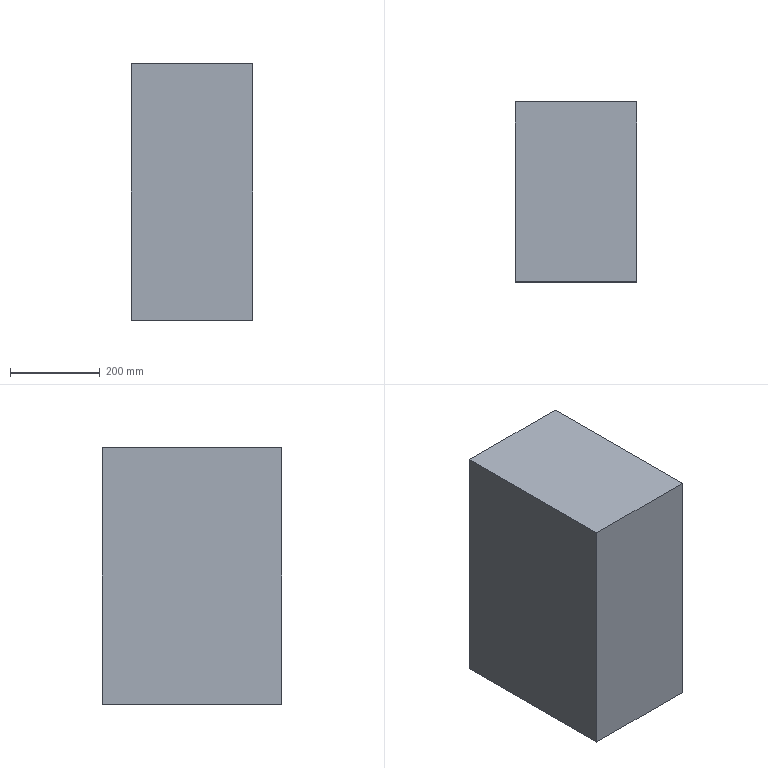Part | STEP file | kunzaxiang | 1 solid | 11 faces | box 270 x 400 x 570 mm | volume 12312000 mm3 | plane 11
STEP:
#1=CARTESIAN_POINT('',(0.,0.,0.));
#2=DIRECTION('',(0.,0.,1.));
#3=DIRECTION('',(1.,0.,0.));
#4=AXIS2_PLACEMENT_3D('',#1,#2,#3);
#5=CARTESIAN_POINT('',(135.,200.,285.));
#6=VERTEX_POINT('',#5);
#7=CARTESIAN_POINT('',(135.,200.,-285.));
#8=VERTEX_POINT('',#7);
#9=CARTESIAN_POINT('',(135.,200.,-285.));
#10=DIRECTION('',(0.,0.,-1.));
#11=VECTOR('',#10,1.);
#12=LINE('',#9,#11);
#13=CARTESIAN_POINT('',(0.,200.,0.));
#14=DIRECTION('',(0.,1.,0.));
#15=DIRECTION('',(0.,0.,1.));
#16=AXIS2_PLACEMENT_3D('',#13,#14,#15);
#17=PLANE('',#16);
#18=CARTESIAN_POINT('',(-285.,135.));
#19=DIRECTION('',(-1.,0.));
#20=VECTOR('',#19,1.);
#21=LINE('',#18,#20);
#22=(GEOMETRIC_REPRESENTATION_CONTEXT(2)PARAMETRIC_REPRESENTATION_CONTEXT()REPRESENTATION_CONTEXT('',''));
#23=DEFINITIONAL_REPRESENTATION('',(#21),#22);
#24=PCURVE('',#17,#23);
#25=CARTESIAN_POINT('',(135.,-200.,-285.));
#26=DIRECTION('',(1.,0.,0.));
#27=DIRECTION('',(0.,0.,-1.));
#28=AXIS2_PLACEMENT_3D('',#25,#26,#27);
#29=PLANE('',#28);
#30=CARTESIAN_POINT('',(0.,400.));
#31=DIRECTION('',(1.,0.));
#32=VECTOR('',#31,1.);
#33=LINE('',#30,#32);
#34=(GEOMETRIC_REPRESENTATION_CONTEXT(2)PARAMETRIC_REPRESENTATION_CONTEXT()REPRESENTATION_CONTEXT('',''));
#35=DEFINITIONAL_REPRESENTATION('',(#33),#34);
#36=PCURVE('',#29,#35);
#37=SURFACE_CURVE('',#12,(#24,#36),.PCURVE_S1.);
#38=EDGE_CURVE('',#6,#8,#37,.T.);
#39=ORIENTED_EDGE('',*,*,#38,.T.);
#40=CARTESIAN_POINT('',(-135.,200.,-285.));
#41=VERTEX_POINT('',#40);
#42=CARTESIAN_POINT('',(-135.,200.,-285.));
#43=DIRECTION('',(-1.,0.,0.));
#44=VECTOR('',#43,1.);
#45=LINE('',#42,#44);
#46=CARTESIAN_POINT('',(-285.,-135.));
#47=DIRECTION('',(0.,-1.));
#48=VECTOR('',#47,1.);
#49=LINE('',#46,#48);
#50=(GEOMETRIC_REPRESENTATION_CONTEXT(2)PARAMETRIC_REPRESENTATION_CONTEXT()REPRESENTATION_CONTEXT('',''));
#51=DEFINITIONAL_REPRESENTATION('',(#49),#50);
#52=PCURVE('',#17,#51);
#53=CARTESIAN_POINT('',(-135.,-200.,-285.));
#54=DIRECTION('',(0.,0.,-1.));
#55=DIRECTION('',(-1.,0.,0.));
#56=AXIS2_PLACEMENT_3D('',#53,#54,#55);
#57=PLANE('',#56);
#58=CARTESIAN_POINT('',(0.,400.));
#59=DIRECTION('',(1.,0.));
#60=VECTOR('',#59,1.);
#61=LINE('',#58,#60);
#62=(GEOMETRIC_REPRESENTATION_CONTEXT(2)PARAMETRIC_REPRESENTATION_CONTEXT()REPRESENTATION_CONTEXT('',''));
#63=DEFINITIONAL_REPRESENTATION('',(#61),#62);
#64=PCURVE('',#57,#63);
#65=SURFACE_CURVE('',#45,(#52,#64),.PCURVE_S1.);
#66=EDGE_CURVE('',#8,#41,#65,.T.);
#67=ORIENTED_EDGE('',*,*,#66,.T.);
#68=CARTESIAN_POINT('',(-135.,200.,285.));
#69=VERTEX_POINT('',#68);
#70=CARTESIAN_POINT('',(-135.,200.,-285.));
#71=DIRECTION('',(0.,0.,1.));
#72=VECTOR('',#71,1.);
#73=LINE('',#70,#72);
#74=CARTESIAN_POINT('',(-285.,-135.));
#75=DIRECTION('',(1.,0.));
#76=VECTOR('',#75,1.);
#77=LINE('',#74,#76);
#78=(GEOMETRIC_REPRESENTATION_CONTEXT(2)PARAMETRIC_REPRESENTATION_CONTEXT()REPRESENTATION_CONTEXT('',''));
#79=DEFINITIONAL_REPRESENTATION('',(#77),#78);
#80=PCURVE('',#17,#79);
#81=CARTESIAN_POINT('',(-135.,-200.,-285.));
#82=DIRECTION('',(-1.,0.,0.));
#83=DIRECTION('',(0.,0.,1.));
#84=AXIS2_PLACEMENT_3D('',#81,#82,#83);
#85=PLANE('',#84);
#86=CARTESIAN_POINT('',(0.,400.));
#87=DIRECTION('',(1.,0.));
#88=VECTOR('',#87,1.);
#89=LINE('',#86,#88);
#90=(GEOMETRIC_REPRESENTATION_CONTEXT(2)PARAMETRIC_REPRESENTATION_CONTEXT()REPRESENTATION_CONTEXT('',''));
#91=DEFINITIONAL_REPRESENTATION('',(#89),#90);
#92=PCURVE('',#85,#91);
#93=SURFACE_CURVE('',#73,(#80,#92),.PCURVE_S1.);
#94=EDGE_CURVE('',#41,#69,#93,.T.);
#95=ORIENTED_EDGE('',*,*,#94,.T.);
#96=CARTESIAN_POINT('',(-135.,200.,285.));
#97=DIRECTION('',(1.,0.,0.));
#98=VECTOR('',#97,1.);
#99=LINE('',#96,#98);
#100=CARTESIAN_POINT('',(285.,-135.));
#101=DIRECTION('',(0.,1.));
#102=VECTOR('',#101,1.);
#103=LINE('',#100,#102);
#104=(GEOMETRIC_REPRESENTATION_CONTEXT(2)PARAMETRIC_REPRESENTATION_CONTEXT()REPRESENTATION_CONTEXT('',''));
#105=DEFINITIONAL_REPRESENTATION('',(#103),#104);
#106=PCURVE('',#17,#105);
#107=CARTESIAN_POINT('',(-135.,-200.,285.));
#108=DIRECTION('',(0.,0.,1.));
#109=DIRECTION('',(1.,0.,0.));
#110=AXIS2_PLACEMENT_3D('',#107,#108,#109);
#111=PLANE('',#110);
#112=CARTESIAN_POINT('',(0.,400.));
#113=DIRECTION('',(1.,0.));
#114=VECTOR('',#113,1.);
#115=LINE('',#112,#114);
#116=(GEOMETRIC_REPRESENTATION_CONTEXT(2)PARAMETRIC_REPRESENTATION_CONTEXT()REPRESENTATION_CONTEXT('',''));
#117=DEFINITIONAL_REPRESENTATION('',(#115),#116);
#118=PCURVE('',#111,#117);
#119=SURFACE_CURVE('',#99,(#106,#118),.PCURVE_S1.);
#120=EDGE_CURVE('',#69,#6,#119,.T.);
#121=ORIENTED_EDGE('',*,*,#120,.T.);
#122=EDGE_LOOP('',(#39,#67,#95,#121));
#123=FACE_BOUND('',#122,.T.);
#124=CARTESIAN_POINT('',(120.,200.,-270.));
#125=VERTEX_POINT('',#124);
#126=CARTESIAN_POINT('',(-120.,200.,-270.));
#127=VERTEX_POINT('',#126);
#128=CARTESIAN_POINT('',(-120.,200.,-270.));
#129=DIRECTION('',(-1.,0.,0.));
#130=VECTOR('',#129,1.);
#131=LINE('',#128,#130);
#132=CARTESIAN_POINT('',(-270.,-120.));
#133=DIRECTION('',(0.,-1.));
#134=VECTOR('',#133,1.);
#135=LINE('',#132,#134);
#136=(GEOMETRIC_REPRESENTATION_CONTEXT(2)PARAMETRIC_REPRESENTATION_CONTEXT()REPRESENTATION_CONTEXT('',''));
#137=DEFINITIONAL_REPRESENTATION('',(#135),#136);
#138=PCURVE('',#17,#137);
#139=CARTESIAN_POINT('',(-120.,200.,-270.));
#140=DIRECTION('',(0.,0.,1.));
#141=DIRECTION('',(1.,0.,0.));
#142=AXIS2_PLACEMENT_3D('',#139,#140,#141);
#143=PLANE('',#142);
#144=CARTESIAN_POINT('',(0.,0.));
#145=DIRECTION('',(-1.,0.));
#146=VECTOR('',#145,1.);
#147=LINE('',#144,#146);
#148=(GEOMETRIC_REPRESENTATION_CONTEXT(2)PARAMETRIC_REPRESENTATION_CONTEXT()REPRESENTATION_CONTEXT('',''));
#149=DEFINITIONAL_REPRESENTATION('',(#147),#148);
#150=PCURVE('',#143,#149);
#151=SURFACE_CURVE('',#131,(#138,#150),.PCURVE_S1.);
#152=EDGE_CURVE('',#125,#127,#151,.T.);
#153=ORIENTED_EDGE('',*,*,#152,.F.);
#154=CARTESIAN_POINT('',(120.,200.,270.));
#155=VERTEX_POINT('',#154);
#156=CARTESIAN_POINT('',(120.,200.,-270.));
#157=DIRECTION('',(0.,0.,-1.));
#158=VECTOR('',#157,1.);
#159=LINE('',#156,#158);
#160=CARTESIAN_POINT('',(-270.,120.));
#161=DIRECTION('',(-1.,0.));
#162=VECTOR('',#161,1.);
#163=LINE('',#160,#162);
#164=(GEOMETRIC_REPRESENTATION_CONTEXT(2)PARAMETRIC_REPRESENTATION_CONTEXT()REPRESENTATION_CONTEXT('',''));
#165=DEFINITIONAL_REPRESENTATION('',(#163),#164);
#166=PCURVE('',#17,#165);
#167=CARTESIAN_POINT('',(120.,200.,-270.));
#168=DIRECTION('',(-1.,0.,0.));
#169=DIRECTION('',(0.,0.,1.));
#170=AXIS2_PLACEMENT_3D('',#167,#168,#169);
#171=PLANE('',#170);
#172=CARTESIAN_POINT('',(0.,0.));
#173=DIRECTION('',(-1.,0.));
#174=VECTOR('',#173,1.);
#175=LINE('',#172,#174);
#176=(GEOMETRIC_REPRESENTATION_CONTEXT(2)PARAMETRIC_REPRESENTATION_CONTEXT()REPRESENTATION_CONTEXT('',''));
#177=DEFINITIONAL_REPRESENTATION('',(#175),#176);
#178=PCURVE('',#171,#177);
#179=SURFACE_CURVE('',#159,(#166,#178),.PCURVE_S1.);
#180=EDGE_CURVE('',#155,#125,#179,.T.);
#181=ORIENTED_EDGE('',*,*,#180,.F.);
#182=CARTESIAN_POINT('',(-120.,200.,270.));
#183=VERTEX_POINT('',#182);
#184=CARTESIAN_POINT('',(-120.,200.,270.));
#185=DIRECTION('',(1.,0.,0.));
#186=VECTOR('',#185,1.);
#187=LINE('',#184,#186);
#188=CARTESIAN_POINT('',(270.,-120.));
#189=DIRECTION('',(0.,1.));
#190=VECTOR('',#189,1.);
#191=LINE('',#188,#190);
#192=(GEOMETRIC_REPRESENTATION_CONTEXT(2)PARAMETRIC_REPRESENTATION_CONTEXT()REPRESENTATION_CONTEXT('',''));
#193=DEFINITIONAL_REPRESENTATION('',(#191),#192);
#194=PCURVE('',#17,#193);
#195=CARTESIAN_POINT('',(-120.,200.,270.));
#196=DIRECTION('',(0.,0.,-1.));
#197=DIRECTION('',(-1.,0.,0.));
#198=AXIS2_PLACEMENT_3D('',#195,#196,#197);
#199=PLANE('',#198);
#200=CARTESIAN_POINT('',(0.,0.));
#201=DIRECTION('',(-1.,0.));
#202=VECTOR('',#201,1.);
#203=LINE('',#200,#202);
#204=(GEOMETRIC_REPRESENTATION_CONTEXT(2)PARAMETRIC_REPRESENTATION_CONTEXT()REPRESENTATION_CONTEXT('',''));
#205=DEFINITIONAL_REPRESENTATION('',(#203),#204);
#206=PCURVE('',#199,#205);
#207=SURFACE_CURVE('',#187,(#194,#206),.PCURVE_S1.);
#208=EDGE_CURVE('',#183,#155,#207,.T.);
#209=ORIENTED_EDGE('',*,*,#208,.F.);
#210=CARTESIAN_POINT('',(-120.,200.,-270.));
#211=DIRECTION('',(0.,0.,1.));
#212=VECTOR('',#211,1.);
#213=LINE('',#210,#212);
#214=CARTESIAN_POINT('',(-270.,-120.));
#215=DIRECTION('',(1.,0.));
#216=VECTOR('',#215,1.);
#217=LINE('',#214,#216);
#218=(GEOMETRIC_REPRESENTATION_CONTEXT(2)PARAMETRIC_REPRESENTATION_CONTEXT()REPRESENTATION_CONTEXT('',''));
#219=DEFINITIONAL_REPRESENTATION('',(#217),#218);
#220=PCURVE('',#17,#219);
#221=CARTESIAN_POINT('',(-120.,200.,-270.));
#222=DIRECTION('',(1.,0.,0.));
#223=DIRECTION('',(0.,0.,-1.));
#224=AXIS2_PLACEMENT_3D('',#221,#222,#223);
#225=PLANE('',#224);
#226=CARTESIAN_POINT('',(0.,0.));
#227=DIRECTION('',(-1.,0.));
#228=VECTOR('',#227,1.);
#229=LINE('',#226,#228);
#230=(GEOMETRIC_REPRESENTATION_CONTEXT(2)PARAMETRIC_REPRESENTATION_CONTEXT()REPRESENTATION_CONTEXT('',''));
#231=DEFINITIONAL_REPRESENTATION('',(#229),#230);
#232=PCURVE('',#225,#231);
#233=SURFACE_CURVE('',#213,(#220,#232),.PCURVE_S1.);
#234=EDGE_CURVE('',#127,#183,#233,.T.);
#235=ORIENTED_EDGE('',*,*,#234,.F.);
#236=EDGE_LOOP('',(#153,#181,#209,#235));
#237=FACE_BOUND('',#236,.T.);
#238=ADVANCED_FACE('',(#123,#237),#17,.T.);
#239=ORIENTED_EDGE('',*,*,#38,.F.);
#240=CARTESIAN_POINT('',(135.,-200.,285.));
#241=VERTEX_POINT('',#240);
#242=CARTESIAN_POINT('',(135.,-200.,285.));
#243=DIRECTION('',(0.,1.,0.));
#244=VECTOR('',#243,1.);
#245=LINE('',#242,#244);
#246=CARTESIAN_POINT('',(-570.,0.));
#247=DIRECTION('',(0.,1.));
#248=VECTOR('',#247,1.);
#249=LINE('',#246,#248);
#250=(GEOMETRIC_REPRESENTATION_CONTEXT(2)PARAMETRIC_REPRESENTATION_CONTEXT()REPRESENTATION_CONTEXT('',''));
#251=DEFINITIONAL_REPRESENTATION('',(#249),#250);
#252=PCURVE('',#29,#251);
#253=CARTESIAN_POINT('',(270.,0.));
#254=DIRECTION('',(0.,1.));
#255=VECTOR('',#254,1.);
#256=LINE('',#253,#255);
#257=(GEOMETRIC_REPRESENTATION_CONTEXT(2)PARAMETRIC_REPRESENTATION_CONTEXT()REPRESENTATION_CONTEXT('',''));
#258=DEFINITIONAL_REPRESENTATION('',(#256),#257);
#259=PCURVE('',#111,#258);
#260=SURFACE_CURVE('',#245,(#252,#259),.PCURVE_S1.);
#261=EDGE_CURVE('',#241,#6,#260,.T.);
#262=ORIENTED_EDGE('',*,*,#261,.F.);
#263=CARTESIAN_POINT('',(135.,-200.,-285.));
#264=VERTEX_POINT('',#263);
#265=CARTESIAN_POINT('',(135.,-200.,-285.));
#266=DIRECTION('',(0.,0.,-1.));
#267=VECTOR('',#266,1.);
#268=LINE('',#265,#267);
#269=CARTESIAN_POINT('',(0.,0.));
#270=DIRECTION('',(1.,0.));
#271=VECTOR('',#270,1.);
#272=LINE('',#269,#271);
#273=(GEOMETRIC_REPRESENTATION_CONTEXT(2)PARAMETRIC_REPRESENTATION_CONTEXT()REPRESENTATION_CONTEXT('',''));
#274=DEFINITIONAL_REPRESENTATION('',(#272),#273);
#275=PCURVE('',#29,#274);
#276=CARTESIAN_POINT('',(0.,-200.,0.));
#277=DIRECTION('',(0.,1.,0.));
#278=DIRECTION('',(0.,0.,1.));
#279=AXIS2_PLACEMENT_3D('',#276,#277,#278);
#280=PLANE('',#279);
#281=CARTESIAN_POINT('',(-285.,135.));
#282=DIRECTION('',(-1.,0.));
#283=VECTOR('',#282,1.);
#284=LINE('',#281,#283);
#285=(GEOMETRIC_REPRESENTATION_CONTEXT(2)PARAMETRIC_REPRESENTATION_CONTEXT()REPRESENTATION_CONTEXT('',''));
#286=DEFINITIONAL_REPRESENTATION('',(#284),#285);
#287=PCURVE('',#280,#286);
#288=SURFACE_CURVE('',#268,(#275,#287),.PCURVE_S1.);
#289=EDGE_CURVE('',#241,#264,#288,.T.);
#290=ORIENTED_EDGE('',*,*,#289,.T.);
#291=CARTESIAN_POINT('',(135.,-200.,-285.));
#292=DIRECTION('',(0.,1.,0.));
#293=VECTOR('',#292,1.);
#294=LINE('',#291,#293);
#295=CARTESIAN_POINT('',(0.,0.));
#296=DIRECTION('',(0.,1.));
#297=VECTOR('',#296,1.);
#298=LINE('',#295,#297);
#299=(GEOMETRIC_REPRESENTATION_CONTEXT(2)PARAMETRIC_REPRESENTATION_CONTEXT()REPRESENTATION_CONTEXT('',''));
#300=DEFINITIONAL_REPRESENTATION('',(#298),#299);
#301=PCURVE('',#29,#300);
#302=CARTESIAN_POINT('',(-270.,0.));
#303=DIRECTION('',(0.,1.));
#304=VECTOR('',#303,1.);
#305=LINE('',#302,#304);
#306=(GEOMETRIC_REPRESENTATION_CONTEXT(2)PARAMETRIC_REPRESENTATION_CONTEXT()REPRESENTATION_CONTEXT('',''));
#307=DEFINITIONAL_REPRESENTATION('',(#305),#306);
#308=PCURVE('',#57,#307);
#309=SURFACE_CURVE('',#294,(#301,#308),.PCURVE_S1.);
#310=EDGE_CURVE('',#264,#8,#309,.T.);
#311=ORIENTED_EDGE('',*,*,#310,.T.);
#312=EDGE_LOOP('',(#239,#262,#290,#311));
#313=FACE_BOUND('',#312,.T.);
#314=ADVANCED_FACE('',(#313),#29,.T.);
#315=ORIENTED_EDGE('',*,*,#120,.F.);
#316=CARTESIAN_POINT('',(-135.,-200.,285.));
#317=VERTEX_POINT('',#316);
#318=CARTESIAN_POINT('',(-135.,-200.,285.));
#319=DIRECTION('',(0.,1.,0.));
#320=VECTOR('',#319,1.);
#321=LINE('',#318,#320);
#322=CARTESIAN_POINT('',(0.,0.));
#323=DIRECTION('',(0.,1.));
#324=VECTOR('',#323,1.);
#325=LINE('',#322,#324);
#326=(GEOMETRIC_REPRESENTATION_CONTEXT(2)PARAMETRIC_REPRESENTATION_CONTEXT()REPRESENTATION_CONTEXT('',''));
#327=DEFINITIONAL_REPRESENTATION('',(#325),#326);
#328=PCURVE('',#111,#327);
#329=CARTESIAN_POINT('',(570.,0.));
#330=DIRECTION('',(0.,1.));
#331=VECTOR('',#330,1.);
#332=LINE('',#329,#331);
#333=(GEOMETRIC_REPRESENTATION_CONTEXT(2)PARAMETRIC_REPRESENTATION_CONTEXT()REPRESENTATION_CONTEXT('',''));
#334=DEFINITIONAL_REPRESENTATION('',(#332),#333);
#335=PCURVE('',#85,#334);
#336=SURFACE_CURVE('',#321,(#328,#335),.PCURVE_S1.);
#337=EDGE_CURVE('',#317,#69,#336,.T.);
#338=ORIENTED_EDGE('',*,*,#337,.F.);
#339=CARTESIAN_POINT('',(-135.,-200.,285.));
#340=DIRECTION('',(1.,0.,0.));
#341=VECTOR('',#340,1.);
#342=LINE('',#339,#341);
#343=CARTESIAN_POINT('',(0.,0.));
#344=DIRECTION('',(1.,0.));
#345=VECTOR('',#344,1.);
#346=LINE('',#343,#345);
#347=(GEOMETRIC_REPRESENTATION_CONTEXT(2)PARAMETRIC_REPRESENTATION_CONTEXT()REPRESENTATION_CONTEXT('',''));
#348=DEFINITIONAL_REPRESENTATION('',(#346),#347);
#349=PCURVE('',#111,#348);
#350=CARTESIAN_POINT('',(285.,-135.));
#351=DIRECTION('',(0.,1.));
#352=VECTOR('',#351,1.);
#353=LINE('',#350,#352);
#354=(GEOMETRIC_REPRESENTATION_CONTEXT(2)PARAMETRIC_REPRESENTATION_CONTEXT()REPRESENTATION_CONTEXT('',''));
#355=DEFINITIONAL_REPRESENTATION('',(#353),#354);
#356=PCURVE('',#280,#355);
#357=SURFACE_CURVE('',#342,(#349,#356),.PCURVE_S1.);
#358=EDGE_CURVE('',#317,#241,#357,.T.);
#359=ORIENTED_EDGE('',*,*,#358,.T.);
#360=ORIENTED_EDGE('',*,*,#261,.T.);
#361=EDGE_LOOP('',(#315,#338,#359,#360));
#362=FACE_BOUND('',#361,.T.);
#363=ADVANCED_FACE('',(#362),#111,.T.);
#364=ORIENTED_EDGE('',*,*,#94,.F.);
#365=CARTESIAN_POINT('',(-135.,-200.,-285.));
#366=VERTEX_POINT('',#365);
#367=CARTESIAN_POINT('',(-135.,-200.,-285.));
#368=DIRECTION('',(0.,1.,0.));
#369=VECTOR('',#368,1.);
#370=LINE('',#367,#369);
#371=CARTESIAN_POINT('',(0.,0.));
#372=DIRECTION('',(0.,1.));
#373=VECTOR('',#372,1.);
#374=LINE('',#371,#373);
#375=(GEOMETRIC_REPRESENTATION_CONTEXT(2)PARAMETRIC_REPRESENTATION_CONTEXT()REPRESENTATION_CONTEXT('',''));
#376=DEFINITIONAL_REPRESENTATION('',(#374),#375);
#377=PCURVE('',#85,#376);
#378=CARTESIAN_POINT('',(0.,0.));
#379=DIRECTION('',(0.,1.));
#380=VECTOR('',#379,1.);
#381=LINE('',#378,#380);
#382=(GEOMETRIC_REPRESENTATION_CONTEXT(2)PARAMETRIC_REPRESENTATION_CONTEXT()REPRESENTATION_CONTEXT('',''));
#383=DEFINITIONAL_REPRESENTATION('',(#381),#382);
#384=PCURVE('',#57,#383);
#385=SURFACE_CURVE('',#370,(#377,#384),.PCURVE_S1.);
#386=EDGE_CURVE('',#366,#41,#385,.T.);
#387=ORIENTED_EDGE('',*,*,#386,.F.);
#388=CARTESIAN_POINT('',(-135.,-200.,-285.));
#389=DIRECTION('',(0.,0.,1.));
#390=VECTOR('',#389,1.);
#391=LINE('',#388,#390);
#392=CARTESIAN_POINT('',(0.,0.));
#393=DIRECTION('',(1.,0.));
#394=VECTOR('',#393,1.);
#395=LINE('',#392,#394);
#396=(GEOMETRIC_REPRESENTATION_CONTEXT(2)PARAMETRIC_REPRESENTATION_CONTEXT()REPRESENTATION_CONTEXT('',''));
#397=DEFINITIONAL_REPRESENTATION('',(#395),#396);
#398=PCURVE('',#85,#397);
#399=CARTESIAN_POINT('',(-285.,-135.));
#400=DIRECTION('',(1.,0.));
#401=VECTOR('',#400,1.);
#402=LINE('',#399,#401);
#403=(GEOMETRIC_REPRESENTATION_CONTEXT(2)PARAMETRIC_REPRESENTATION_CONTEXT()REPRESENTATION_CONTEXT('',''));
#404=DEFINITIONAL_REPRESENTATION('',(#402),#403);
#405=PCURVE('',#280,#404);
#406=SURFACE_CURVE('',#391,(#398,#405),.PCURVE_S1.);
#407=EDGE_CURVE('',#366,#317,#406,.T.);
#408=ORIENTED_EDGE('',*,*,#407,.T.);
#409=ORIENTED_EDGE('',*,*,#337,.T.);
#410=EDGE_LOOP('',(#364,#387,#408,#409));
#411=FACE_BOUND('',#410,.T.);
#412=ADVANCED_FACE('',(#411),#85,.T.);
#413=ORIENTED_EDGE('',*,*,#66,.F.);
#414=ORIENTED_EDGE('',*,*,#310,.F.);
#415=CARTESIAN_POINT('',(-135.,-200.,-285.));
#416=DIRECTION('',(-1.,0.,0.));
#417=VECTOR('',#416,1.);
#418=LINE('',#415,#417);
#419=CARTESIAN_POINT('',(0.,0.));
#420=DIRECTION('',(1.,0.));
#421=VECTOR('',#420,1.);
#422=LINE('',#419,#421);
#423=(GEOMETRIC_REPRESENTATION_CONTEXT(2)PARAMETRIC_REPRESENTATION_CONTEXT()REPRESENTATION_CONTEXT('',''));
#424=DEFINITIONAL_REPRESENTATION('',(#422),#423);
#425=PCURVE('',#57,#424);
#426=CARTESIAN_POINT('',(-285.,-135.));
#427=DIRECTION('',(0.,-1.));
#428=VECTOR('',#427,1.);
#429=LINE('',#426,#428);
#430=(GEOMETRIC_REPRESENTATION_CONTEXT(2)PARAMETRIC_REPRESENTATION_CONTEXT()REPRESENTATION_CONTEXT('',''));
#431=DEFINITIONAL_REPRESENTATION('',(#429),#430);
#432=PCURVE('',#280,#431);
#433=SURFACE_CURVE('',#418,(#425,#432),.PCURVE_S1.);
#434=EDGE_CURVE('',#264,#366,#433,.T.);
#435=ORIENTED_EDGE('',*,*,#434,.T.);
#436=ORIENTED_EDGE('',*,*,#386,.T.);
#437=EDGE_LOOP('',(#413,#414,#435,#436));
#438=FACE_BOUND('',#437,.T.);
#439=ADVANCED_FACE('',(#438),#57,.T.);
#440=ORIENTED_EDGE('',*,*,#289,.F.);
#441=ORIENTED_EDGE('',*,*,#358,.F.);
#442=ORIENTED_EDGE('',*,*,#407,.F.);
#443=ORIENTED_EDGE('',*,*,#434,.F.);
#444=EDGE_LOOP('',(#440,#441,#442,#443));
#445=FACE_BOUND('',#444,.T.);
#446=ADVANCED_FACE('',(#445),#280,.F.);
#447=CARTESIAN_POINT('',(120.,-180.,270.));
#448=VERTEX_POINT('',#447);
#449=CARTESIAN_POINT('',(120.,200.,270.));
#450=DIRECTION('',(0.,-1.,0.));
#451=VECTOR('',#450,1.);
#452=LINE('',#449,#451);
#453=CARTESIAN_POINT('',(540.,0.));
#454=DIRECTION('',(0.,-1.));
#455=VECTOR('',#454,1.);
#456=LINE('',#453,#455);
#457=(GEOMETRIC_REPRESENTATION_CONTEXT(2)PARAMETRIC_REPRESENTATION_CONTEXT()REPRESENTATION_CONTEXT('',''));
#458=DEFINITIONAL_REPRESENTATION('',(#456),#457);
#459=PCURVE('',#171,#458);
#460=CARTESIAN_POINT('',(-240.,0.));
#461=DIRECTION('',(0.,-1.));
#462=VECTOR('',#461,1.);
#463=LINE('',#460,#462);
#464=(GEOMETRIC_REPRESENTATION_CONTEXT(2)PARAMETRIC_REPRESENTATION_CONTEXT()REPRESENTATION_CONTEXT('',''));
#465=DEFINITIONAL_REPRESENTATION('',(#463),#464);
#466=PCURVE('',#199,#465);
#467=SURFACE_CURVE('',#452,(#459,#466),.PCURVE_S1.);
#468=EDGE_CURVE('',#155,#448,#467,.T.);
#469=ORIENTED_EDGE('',*,*,#468,.F.);
#470=ORIENTED_EDGE('',*,*,#180,.T.);
#471=CARTESIAN_POINT('',(120.,-180.,-270.));
#472=VERTEX_POINT('',#471);
#473=CARTESIAN_POINT('',(120.,200.,-270.));
#474=DIRECTION('',(0.,-1.,0.));
#475=VECTOR('',#474,1.);
#476=LINE('',#473,#475);
#477=CARTESIAN_POINT('',(0.,0.));
#478=DIRECTION('',(0.,-1.));
#479=VECTOR('',#478,1.);
#480=LINE('',#477,#479);
#481=(GEOMETRIC_REPRESENTATION_CONTEXT(2)PARAMETRIC_REPRESENTATION_CONTEXT()REPRESENTATION_CONTEXT('',''));
#482=DEFINITIONAL_REPRESENTATION('',(#480),#481);
#483=PCURVE('',#171,#482);
#484=CARTESIAN_POINT('',(240.,0.));
#485=DIRECTION('',(0.,-1.));
#486=VECTOR('',#485,1.);
#487=LINE('',#484,#486);
#488=(GEOMETRIC_REPRESENTATION_CONTEXT(2)PARAMETRIC_REPRESENTATION_CONTEXT()REPRESENTATION_CONTEXT('',''));
#489=DEFINITIONAL_REPRESENTATION('',(#487),#488);
#490=PCURVE('',#143,#489);
#491=SURFACE_CURVE('',#476,(#483,#490),.PCURVE_S1.);
#492=EDGE_CURVE('',#125,#472,#491,.T.);
#493=ORIENTED_EDGE('',*,*,#492,.T.);
#494=CARTESIAN_POINT('',(120.,-180.,-270.));
#495=DIRECTION('',(0.,0.,-1.));
#496=VECTOR('',#495,1.);
#497=LINE('',#494,#496);
#498=CARTESIAN_POINT('',(0.,-380.));
#499=DIRECTION('',(-1.,0.));
#500=VECTOR('',#499,1.);
#501=LINE('',#498,#500);
#502=(GEOMETRIC_REPRESENTATION_CONTEXT(2)PARAMETRIC_REPRESENTATION_CONTEXT()REPRESENTATION_CONTEXT('',''));
#503=DEFINITIONAL_REPRESENTATION('',(#501),#502);
#504=PCURVE('',#171,#503);
#505=CARTESIAN_POINT('',(0.,-180.,0.));
#506=DIRECTION('',(0.,1.,0.));
#507=DIRECTION('',(0.,0.,1.));
#508=AXIS2_PLACEMENT_3D('',#505,#506,#507);
#509=PLANE('',#508);
#510=CARTESIAN_POINT('',(-270.,120.));
#511=DIRECTION('',(-1.,0.));
#512=VECTOR('',#511,1.);
#513=LINE('',#510,#512);
#514=(GEOMETRIC_REPRESENTATION_CONTEXT(2)PARAMETRIC_REPRESENTATION_CONTEXT()REPRESENTATION_CONTEXT('',''));
#515=DEFINITIONAL_REPRESENTATION('',(#513),#514);
#516=PCURVE('',#509,#515);
#517=SURFACE_CURVE('',#497,(#504,#516),.PCURVE_S1.);
#518=EDGE_CURVE('',#448,#472,#517,.T.);
#519=ORIENTED_EDGE('',*,*,#518,.F.);
#520=EDGE_LOOP('',(#469,#470,#493,#519));
#521=FACE_BOUND('',#520,.T.);
#522=ADVANCED_FACE('',(#521),#171,.T.);
#523=ORIENTED_EDGE('',*,*,#492,.F.);
#524=ORIENTED_EDGE('',*,*,#152,.T.);
#525=CARTESIAN_POINT('',(-120.,-180.,-270.));
#526=VERTEX_POINT('',#525);
#527=CARTESIAN_POINT('',(-120.,200.,-270.));
#528=DIRECTION('',(0.,-1.,0.));
#529=VECTOR('',#528,1.);
#530=LINE('',#527,#529);
#531=CARTESIAN_POINT('',(0.,0.));
#532=DIRECTION('',(0.,-1.));
#533=VECTOR('',#532,1.);
#534=LINE('',#531,#533);
#535=(GEOMETRIC_REPRESENTATION_CONTEXT(2)PARAMETRIC_REPRESENTATION_CONTEXT()REPRESENTATION_CONTEXT('',''));
#536=DEFINITIONAL_REPRESENTATION('',(#534),#535);
#537=PCURVE('',#143,#536);
#538=CARTESIAN_POINT('',(0.,0.));
#539=DIRECTION('',(0.,-1.));
#540=VECTOR('',#539,1.);
#541=LINE('',#538,#540);
#542=(GEOMETRIC_REPRESENTATION_CONTEXT(2)PARAMETRIC_REPRESENTATION_CONTEXT()REPRESENTATION_CONTEXT('',''));
#543=DEFINITIONAL_REPRESENTATION('',(#541),#542);
#544=PCURVE('',#225,#543);
#545=SURFACE_CURVE('',#530,(#537,#544),.PCURVE_S1.);
#546=EDGE_CURVE('',#127,#526,#545,.T.);
#547=ORIENTED_EDGE('',*,*,#546,.T.);
#548=CARTESIAN_POINT('',(-120.,-180.,-270.));
#549=DIRECTION('',(-1.,0.,0.));
#550=VECTOR('',#549,1.);
#551=LINE('',#548,#550);
#552=CARTESIAN_POINT('',(0.,-380.));
#553=DIRECTION('',(-1.,0.));
#554=VECTOR('',#553,1.);
#555=LINE('',#552,#554);
#556=(GEOMETRIC_REPRESENTATION_CONTEXT(2)PARAMETRIC_REPRESENTATION_CONTEXT()REPRESENTATION_CONTEXT('',''));
#557=DEFINITIONAL_REPRESENTATION('',(#555),#556);
#558=PCURVE('',#143,#557);
#559=CARTESIAN_POINT('',(-270.,-120.));
#560=DIRECTION('',(0.,-1.));
#561=VECTOR('',#560,1.);
#562=LINE('',#559,#561);
#563=(GEOMETRIC_REPRESENTATION_CONTEXT(2)PARAMETRIC_REPRESENTATION_CONTEXT()REPRESENTATION_CONTEXT('',''));
#564=DEFINITIONAL_REPRESENTATION('',(#562),#563);
#565=PCURVE('',#509,#564);
#566=SURFACE_CURVE('',#551,(#558,#565),.PCURVE_S1.);
#567=EDGE_CURVE('',#472,#526,#566,.T.);
#568=ORIENTED_EDGE('',*,*,#567,.F.);
#569=EDGE_LOOP('',(#523,#524,#547,#568));
#570=FACE_BOUND('',#569,.T.);
#571=ADVANCED_FACE('',(#570),#143,.T.);
#572=ORIENTED_EDGE('',*,*,#546,.F.);
#573=ORIENTED_EDGE('',*,*,#234,.T.);
#574=CARTESIAN_POINT('',(-120.,-180.,270.));
#575=VERTEX_POINT('',#574);
#576=CARTESIAN_POINT('',(-120.,200.,270.));
#577=DIRECTION('',(0.,-1.,0.));
#578=VECTOR('',#577,1.);
#579=LINE('',#576,#578);
#580=CARTESIAN_POINT('',(-540.,0.));
#581=DIRECTION('',(0.,-1.));
#582=VECTOR('',#581,1.);
#583=LINE('',#580,#582);
#584=(GEOMETRIC_REPRESENTATION_CONTEXT(2)PARAMETRIC_REPRESENTATION_CONTEXT()REPRESENTATION_CONTEXT('',''));
#585=DEFINITIONAL_REPRESENTATION('',(#583),#584);
#586=PCURVE('',#225,#585);
#587=CARTESIAN_POINT('',(0.,0.));
#588=DIRECTION('',(0.,-1.));
#589=VECTOR('',#588,1.);
#590=LINE('',#587,#589);
#591=(GEOMETRIC_REPRESENTATION_CONTEXT(2)PARAMETRIC_REPRESENTATION_CONTEXT()REPRESENTATION_CONTEXT('',''));
#592=DEFINITIONAL_REPRESENTATION('',(#590),#591);
#593=PCURVE('',#199,#592);
#594=SURFACE_CURVE('',#579,(#586,#593),.PCURVE_S1.);
#595=EDGE_CURVE('',#183,#575,#594,.T.);
#596=ORIENTED_EDGE('',*,*,#595,.T.);
#597=CARTESIAN_POINT('',(-120.,-180.,-270.));
#598=DIRECTION('',(0.,0.,1.));
#599=VECTOR('',#598,1.);
#600=LINE('',#597,#599);
#601=CARTESIAN_POINT('',(0.,-380.));
#602=DIRECTION('',(-1.,0.));
#603=VECTOR('',#602,1.);
#604=LINE('',#601,#603);
#605=(GEOMETRIC_REPRESENTATION_CONTEXT(2)PARAMETRIC_REPRESENTATION_CONTEXT()REPRESENTATION_CONTEXT('',''));
#606=DEFINITIONAL_REPRESENTATION('',(#604),#605);
#607=PCURVE('',#225,#606);
#608=CARTESIAN_POINT('',(-270.,-120.));
#609=DIRECTION('',(1.,0.));
#610=VECTOR('',#609,1.);
#611=LINE('',#608,#610);
#612=(GEOMETRIC_REPRESENTATION_CONTEXT(2)PARAMETRIC_REPRESENTATION_CONTEXT()REPRESENTATION_CONTEXT('',''));
#613=DEFINITIONAL_REPRESENTATION('',(#611),#612);
#614=PCURVE('',#509,#613);
#615=SURFACE_CURVE('',#600,(#607,#614),.PCURVE_S1.);
#616=EDGE_CURVE('',#526,#575,#615,.T.);
#617=ORIENTED_EDGE('',*,*,#616,.F.);
#618=EDGE_LOOP('',(#572,#573,#596,#617));
#619=FACE_BOUND('',#618,.T.);
#620=ADVANCED_FACE('',(#619),#225,.T.);
#621=ORIENTED_EDGE('',*,*,#595,.F.);
#622=ORIENTED_EDGE('',*,*,#208,.T.);
#623=ORIENTED_EDGE('',*,*,#468,.T.);
#624=CARTESIAN_POINT('',(-120.,-180.,270.));
#625=DIRECTION('',(1.,0.,0.));
#626=VECTOR('',#625,1.);
#627=LINE('',#624,#626);
#628=CARTESIAN_POINT('',(0.,-380.));
#629=DIRECTION('',(-1.,0.));
#630=VECTOR('',#629,1.);
#631=LINE('',#628,#630);
#632=(GEOMETRIC_REPRESENTATION_CONTEXT(2)PARAMETRIC_REPRESENTATION_CONTEXT()REPRESENTATION_CONTEXT('',''));
#633=DEFINITIONAL_REPRESENTATION('',(#631),#632);
#634=PCURVE('',#199,#633);
#635=CARTESIAN_POINT('',(270.,-120.));
#636=DIRECTION('',(0.,1.));
#637=VECTOR('',#636,1.);
#638=LINE('',#635,#637);
#639=(GEOMETRIC_REPRESENTATION_CONTEXT(2)PARAMETRIC_REPRESENTATION_CONTEXT()REPRESENTATION_CONTEXT('',''));
#640=DEFINITIONAL_REPRESENTATION('',(#638),#639);
#641=PCURVE('',#509,#640);
#642=SURFACE_CURVE('',#627,(#634,#641),.PCURVE_S1.);
#643=EDGE_CURVE('',#575,#448,#642,.T.);
#644=ORIENTED_EDGE('',*,*,#643,.F.);
#645=EDGE_LOOP('',(#621,#622,#623,#644));
#646=FACE_BOUND('',#645,.T.);
#647=ADVANCED_FACE('',(#646),#199,.T.);
#648=ORIENTED_EDGE('',*,*,#518,.T.);
#649=ORIENTED_EDGE('',*,*,#567,.T.);
#650=ORIENTED_EDGE('',*,*,#616,.T.);
#651=ORIENTED_EDGE('',*,*,#643,.T.);
#652=EDGE_LOOP('',(#648,#649,#650,#651));
#653=FACE_BOUND('',#652,.T.);
#654=ADVANCED_FACE('',(#653),#509,.T.);
#655=CLOSED_SHELL('',(#238,#314,#363,#412,#439,#446,#522,#571,#620,#647,#654));
#656=MANIFOLD_SOLID_BREP('',#655);
#657=(LENGTH_UNIT()NAMED_UNIT(*)SI_UNIT(.MILLI.,.METRE.));
#658=UNCERTAINTY_MEASURE_WITH_UNIT(LENGTH_MEASURE(0.0000001),#657,'','');
#659=(NAMED_UNIT(*)PLANE_ANGLE_UNIT()SI_UNIT($,.RADIAN.));
#660=(NAMED_UNIT(*)SI_UNIT($,.STERADIAN.)SOLID_ANGLE_UNIT());
#661=(GEOMETRIC_REPRESENTATION_CONTEXT(3)GLOBAL_UNCERTAINTY_ASSIGNED_CONTEXT((#658))GLOBAL_UNIT_ASSIGNED_CONTEXT((#657,#659,#660))REPRESENTATION_CONTEXT('',''));
#662=ADVANCED_BREP_SHAPE_REPRESENTATION('',(#4,#656),#661);